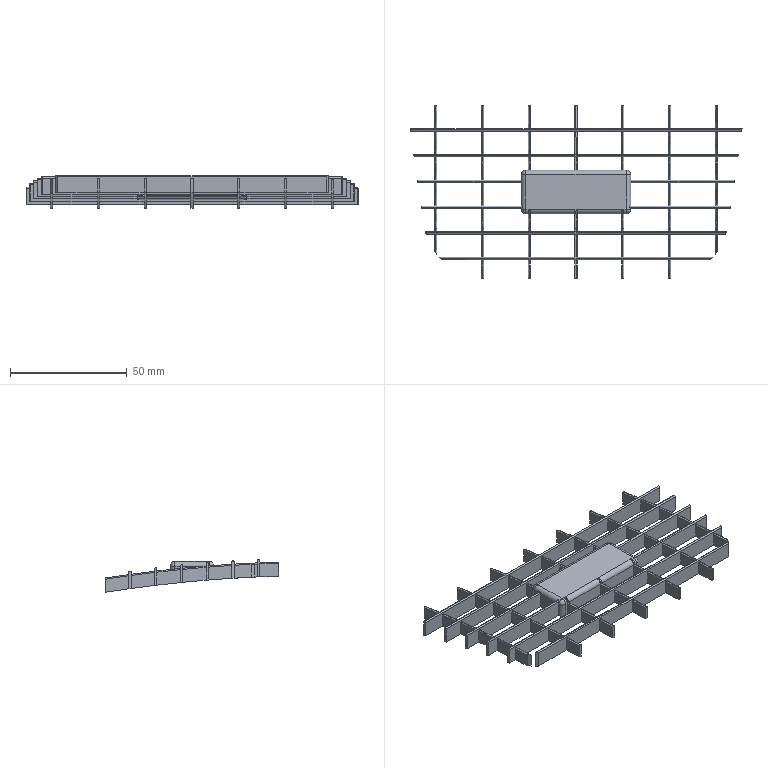Part | SolidWorks | features SplitBody 1 | 1 solid | 294 faces | box 141.922 x 74 x 13.927 mm | volume 14904 mm3 | plane 134 | spline 117 | cylinder 39 | sphere 4 | commonest cylinder face diameters 1 x16 4 x11 54 x8 1174 x4